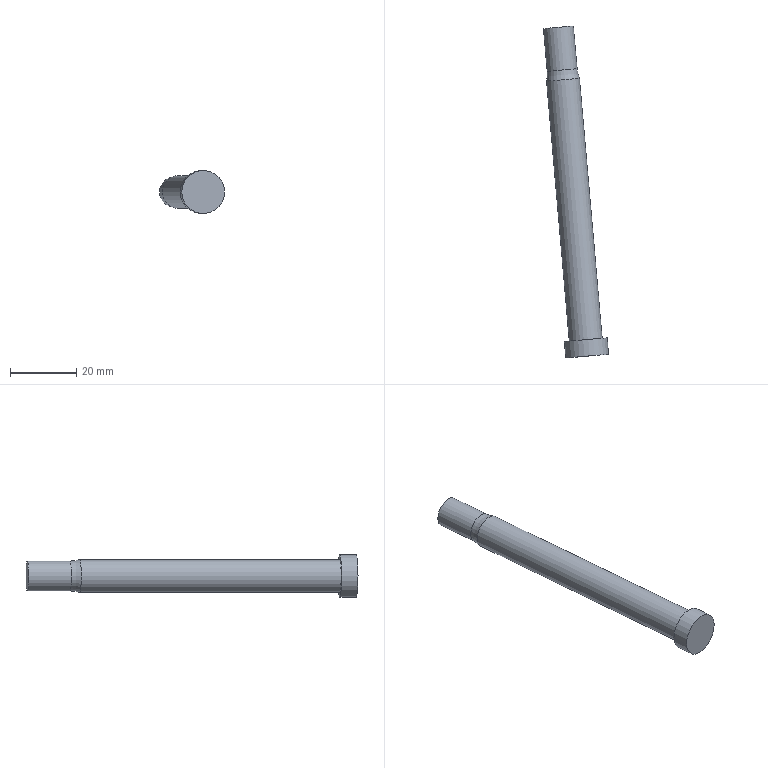Part | NX | features SPAS 10-80-9.100 2 | 1 solid | 7 faces | box 19.724 x 100.583 x 13 mm | volume 7922 mm3 | plane 3 | cylinder 3 | torus 1 | commonest cylinder face diameters 9.1 x1 10 x1 13 x1
STEP:
#1=CARTESIAN_POINT('',(762.749,-44.217,-42.474));
#2=VERTEX_POINT('',#1);
#3=CARTESIAN_POINT('',(758.216,-44.614,-42.474));
#4=DIRECTION('',(0.08716,-0.9962,0.));
#5=DIRECTION('',(0.9962,0.08716,0.));
#6=AXIS2_PLACEMENT_3D('',#3,#4,#5);
#7=CIRCLE('',#6,4.55);
#8=EDGE_CURVE('',#2,#2,#7,.T.);
#9=ORIENTED_EDGE('',*,*,#8,.F.);
#10=EDGE_LOOP('',(#9));
#11=FACE_BOUND('',#10,.T.);
#12=CARTESIAN_POINT('',(758.216,-44.614,-42.474));
#13=DIRECTION('',(-0.08716,0.9962,0.));
#14=DIRECTION('',(-0.9962,-0.08716,0.));
#15=AXIS2_PLACEMENT_3D('',#12,#13,#14);
#16=PLANE('',#15);
#17=ADVANCED_FACE('',(#11),#16,.T.);
#18=CARTESIAN_POINT('',(763.882,-57.168,-42.474));
#19=VERTEX_POINT('',#18);
#20=CARTESIAN_POINT('',(759.349,-57.564,-42.474));
#21=DIRECTION('',(0.08716,-0.9962,0.));
#22=DIRECTION('',(0.9962,0.08716,0.));
#23=AXIS2_PLACEMENT_3D('',#20,#21,#22);
#24=CIRCLE('',#23,4.55);
#25=EDGE_CURVE('',#19,#19,#24,.F.);
#26=ORIENTED_EDGE('',*,*,#25,.T.);
#27=EDGE_LOOP('',(#26));
#28=FACE_BOUND('',#27,.T.);
#29=ORIENTED_EDGE('',*,*,#8,.T.);
#30=EDGE_LOOP('',(#29));
#31=FACE_BOUND('',#30,.T.);
#32=CARTESIAN_POINT('',(758.216,-44.614,-42.474));
#33=DIRECTION('',(0.08716,-0.9962,0.));
#34=DIRECTION('',(0.9962,0.08716,0.));
#35=AXIS2_PLACEMENT_3D('',#32,#33,#34);
#36=CYLINDRICAL_SURFACE('',#35,4.55);
#37=ADVANCED_FACE('',(#28,#31),#36,.T.);
#38=CARTESIAN_POINT('',(761.515,-139.688,-42.474));
#39=VERTEX_POINT('',#38);
#40=CARTESIAN_POINT('',(766.496,-139.252,-42.474));
#41=DIRECTION('',(-0.08716,0.9962,0.));
#42=DIRECTION('',(-0.9962,-0.08716,0.));
#43=AXIS2_PLACEMENT_3D('',#40,#41,#42);
#44=CIRCLE('',#43,5.);
#45=EDGE_CURVE('',#39,#39,#44,.F.);
#46=ORIENTED_EDGE('',*,*,#45,.F.);
#47=EDGE_LOOP('',(#46));
#48=FACE_BOUND('',#47,.T.);
#49=CARTESIAN_POINT('',(764.589,-60.083,-42.474));
#50=VERTEX_POINT('',#49);
#51=CARTESIAN_POINT('',(759.608,-60.519,-42.474));
#52=DIRECTION('',(0.08716,-0.9962,0.));
#53=DIRECTION('',(0.9962,0.08716,0.));
#54=AXIS2_PLACEMENT_3D('',#51,#52,#53);
#55=CIRCLE('',#54,5.);
#56=EDGE_CURVE('',#50,#50,#55,.T.);
#57=ORIENTED_EDGE('',*,*,#56,.T.);
#58=EDGE_LOOP('',(#57));
#59=FACE_BOUND('',#58,.T.);
#60=CARTESIAN_POINT('',(759.608,-60.519,-42.474));
#61=DIRECTION('',(0.08716,-0.9962,0.));
#62=DIRECTION('',(0.9962,0.08716,0.));
#63=AXIS2_PLACEMENT_3D('',#60,#61,#62);
#64=CYLINDRICAL_SURFACE('',#63,5.);
#65=ADVANCED_FACE('',(#48,#59),#64,.T.);
#66=CARTESIAN_POINT('',(773.407,-143.667,-42.474));
#67=VERTEX_POINT('',#66);
#68=CARTESIAN_POINT('',(766.932,-144.233,-42.474));
#69=DIRECTION('',(0.08716,-0.9962,0.));
#70=DIRECTION('',(0.9962,0.08716,0.));
#71=AXIS2_PLACEMENT_3D('',#68,#69,#70);
#72=CIRCLE('',#71,6.5);
#73=EDGE_CURVE('',#67,#67,#72,.F.);
#74=ORIENTED_EDGE('',*,*,#73,.F.);
#75=EDGE_LOOP('',(#74));
#76=FACE_BOUND('',#75,.T.);
#77=CARTESIAN_POINT('',(766.932,-144.233,-42.474));
#78=DIRECTION('',(0.08716,-0.9962,0.));
#79=DIRECTION('',(0.9962,0.08716,0.));
#80=AXIS2_PLACEMENT_3D('',#77,#78,#79);
#81=PLANE('',#80);
#82=ADVANCED_FACE('',(#76),#81,.T.);
#83=ORIENTED_EDGE('',*,*,#45,.T.);
#84=EDGE_LOOP('',(#83));
#85=FACE_BOUND('',#84,.T.);
#86=CARTESIAN_POINT('',(760.021,-139.819,-42.474));
#87=VERTEX_POINT('',#86);
#88=CARTESIAN_POINT('',(766.496,-139.252,-42.474));
#89=DIRECTION('',(-0.08716,0.9962,0.));
#90=DIRECTION('',(-0.9962,-0.08716,0.));
#91=AXIS2_PLACEMENT_3D('',#88,#89,#90);
#92=CIRCLE('',#91,6.5);
#93=EDGE_CURVE('',#87,#87,#92,.F.);
#94=ORIENTED_EDGE('',*,*,#93,.F.);
#95=EDGE_LOOP('',(#94));
#96=FACE_BOUND('',#95,.T.);
#97=CARTESIAN_POINT('',(766.496,-139.252,-42.474));
#98=DIRECTION('',(-0.08716,0.9962,0.));
#99=DIRECTION('',(-0.9962,-0.08716,0.));
#100=AXIS2_PLACEMENT_3D('',#97,#98,#99);
#101=PLANE('',#100);
#102=ADVANCED_FACE('',(#85,#96),#101,.T.);
#103=ORIENTED_EDGE('',*,*,#73,.T.);
#104=EDGE_LOOP('',(#103));
#105=FACE_BOUND('',#104,.T.);
#106=ORIENTED_EDGE('',*,*,#93,.T.);
#107=EDGE_LOOP('',(#106));
#108=FACE_BOUND('',#107,.T.);
#109=CARTESIAN_POINT('',(764.753,-119.328,-42.474));
#110=DIRECTION('',(0.08716,-0.9962,0.));
#111=DIRECTION('',(0.9962,0.08716,0.));
#112=AXIS2_PLACEMENT_3D('',#109,#110,#111);
#113=CYLINDRICAL_SURFACE('',#112,6.5);
#114=ADVANCED_FACE('',(#105,#108),#113,.T.);
#115=ORIENTED_EDGE('',*,*,#25,.F.);
#116=EDGE_LOOP('',(#115));
#117=FACE_BOUND('',#116,.T.);
#118=ORIENTED_EDGE('',*,*,#56,.F.);
#119=EDGE_LOOP('',(#118));
#120=FACE_BOUND('',#119,.T.);
#121=CARTESIAN_POINT('',(759.349,-57.564,-42.474));
#122=DIRECTION('',(0.08716,-0.9962,0.));
#123=DIRECTION('',(0.9962,0.08716,0.));
#124=AXIS2_PLACEMENT_3D('',#121,#122,#123);
#125=TOROIDAL_SURFACE('',#124,14.55,10.);
#126=ADVANCED_FACE('',(#117,#120),#125,.F.);
#127=CLOSED_SHELL('',(#17,#37,#65,#82,#102,#114,#126));
#128=MANIFOLD_SOLID_BREP('',#127);
#129=(LENGTH_UNIT()NAMED_UNIT(*)SI_UNIT(.MILLI.,.METRE.));
#130=UNCERTAINTY_MEASURE_WITH_UNIT(LENGTH_MEASURE(0.00001),#129,'','');
#131=(NAMED_UNIT(*)PLANE_ANGLE_UNIT()SI_UNIT($,.RADIAN.));
#132=(NAMED_UNIT(*)SI_UNIT($,.STERADIAN.)SOLID_ANGLE_UNIT());
#133=(GEOMETRIC_REPRESENTATION_CONTEXT(3)GLOBAL_UNCERTAINTY_ASSIGNED_CONTEXT((#130))GLOBAL_UNIT_ASSIGNED_CONTEXT((#129,#131,#132))REPRESENTATION_CONTEXT('',''));
#134=ADVANCED_BREP_SHAPE_REPRESENTATION('',(#128),#133);